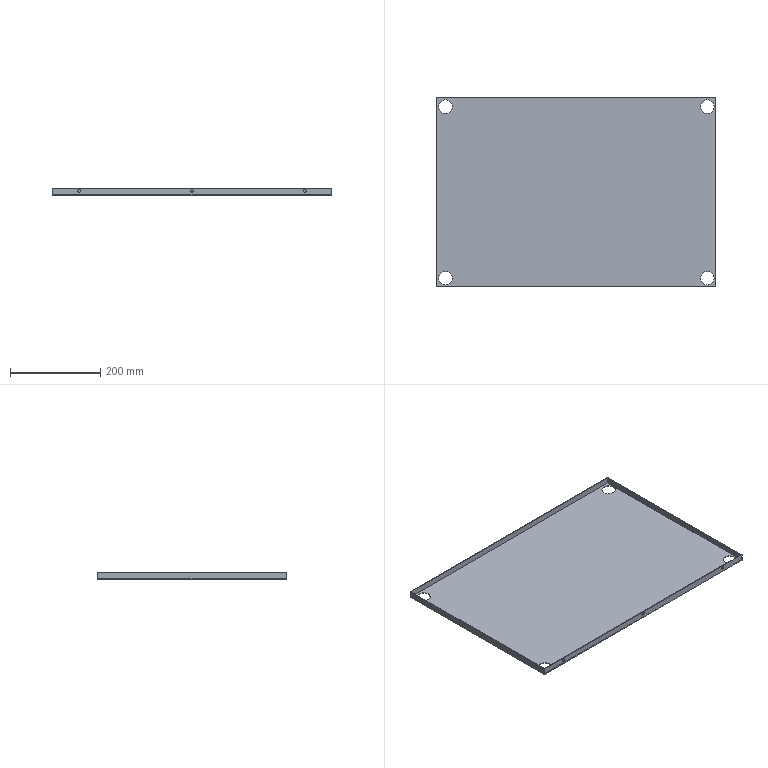Part | SolidWorks | features BaseBody 1 | 1 solid | 25 faces | box 620 x 420 x 15 mm | volume 428208 mm3 | cylinder 14 | plane 11 | commonest cylinder face diameters 30 x8 6.5 x6
STEP:
#1=CARTESIAN_POINT('',(437.517,75.647,0.));
#2=VERTEX_POINT('',#1);
#3=CARTESIAN_POINT('',(467.517,75.647,0.));
#4=VERTEX_POINT('',#3);
#5=CARTESIAN_POINT('',(452.517,75.647,0.));
#6=DIRECTION('',(0.,0.,1.));
#7=DIRECTION('',(1.,0.,0.));
#8=AXIS2_PLACEMENT_3D('',#5,#6,#7);
#9=CIRCLE('',#8,15.);
#10=EDGE_CURVE('',#2,#4,#9,.T.);
#11=ORIENTED_EDGE('',*,*,#10,.F.);
#12=CARTESIAN_POINT('',(437.517,75.647,1.5));
#13=VERTEX_POINT('',#12);
#14=CARTESIAN_POINT('',(437.517,75.647,0.));
#15=DIRECTION('',(0.,0.,1.));
#16=VECTOR('',#15,1000.);
#17=LINE('',#14,#16);
#18=EDGE_CURVE('',#2,#13,#17,.T.);
#19=ORIENTED_EDGE('',*,*,#18,.T.);
#20=CARTESIAN_POINT('',(467.517,75.647,1.5));
#21=VERTEX_POINT('',#20);
#22=CARTESIAN_POINT('',(452.517,75.647,1.5));
#23=DIRECTION('',(0.,0.,-1.));
#24=DIRECTION('',(1.,0.,0.));
#25=AXIS2_PLACEMENT_3D('',#22,#23,#24);
#26=CIRCLE('',#25,15.);
#27=EDGE_CURVE('',#21,#13,#26,.T.);
#28=ORIENTED_EDGE('',*,*,#27,.F.);
#29=CARTESIAN_POINT('',(467.517,75.647,0.));
#30=DIRECTION('',(0.,0.,1.));
#31=VECTOR('',#30,1000.);
#32=LINE('',#29,#31);
#33=EDGE_CURVE('',#4,#21,#32,.T.);
#34=ORIENTED_EDGE('',*,*,#33,.F.);
#35=EDGE_LOOP('',(#11,#19,#28,#34));
#36=FACE_OUTER_BOUND('',#35,.T.);
#37=CARTESIAN_POINT('',(452.517,75.647,0.));
#38=DIRECTION('',(0.,0.,1.));
#39=DIRECTION('',(1.,0.,0.));
#40=AXIS2_PLACEMENT_3D('',#37,#38,#39);
#41=CYLINDRICAL_SURFACE('',#40,15.);
#42=ADVANCED_FACE('',(#36),#41,.F.);
#43=CARTESIAN_POINT('',(-142.483,75.647,0.));
#44=VERTEX_POINT('',#43);
#45=CARTESIAN_POINT('',(-112.483,75.647,0.));
#46=VERTEX_POINT('',#45);
#47=CARTESIAN_POINT('',(-127.483,75.647,0.));
#48=DIRECTION('',(0.,0.,1.));
#49=DIRECTION('',(1.,0.,0.));
#50=AXIS2_PLACEMENT_3D('',#47,#48,#49);
#51=CIRCLE('',#50,15.);
#52=EDGE_CURVE('',#44,#46,#51,.T.);
#53=ORIENTED_EDGE('',*,*,#52,.F.);
#54=CARTESIAN_POINT('',(-142.483,75.647,1.5));
#55=VERTEX_POINT('',#54);
#56=CARTESIAN_POINT('',(-142.483,75.647,0.));
#57=DIRECTION('',(0.,0.,1.));
#58=VECTOR('',#57,1000.);
#59=LINE('',#56,#58);
#60=EDGE_CURVE('',#44,#55,#59,.T.);
#61=ORIENTED_EDGE('',*,*,#60,.T.);
#62=CARTESIAN_POINT('',(-112.483,75.647,1.5));
#63=VERTEX_POINT('',#62);
#64=CARTESIAN_POINT('',(-127.483,75.647,1.5));
#65=DIRECTION('',(0.,0.,-1.));
#66=DIRECTION('',(1.,0.,0.));
#67=AXIS2_PLACEMENT_3D('',#64,#65,#66);
#68=CIRCLE('',#67,15.);
#69=EDGE_CURVE('',#63,#55,#68,.T.);
#70=ORIENTED_EDGE('',*,*,#69,.F.);
#71=CARTESIAN_POINT('',(-112.483,75.647,0.));
#72=DIRECTION('',(0.,0.,1.));
#73=VECTOR('',#72,1000.);
#74=LINE('',#71,#73);
#75=EDGE_CURVE('',#46,#63,#74,.T.);
#76=ORIENTED_EDGE('',*,*,#75,.F.);
#77=EDGE_LOOP('',(#53,#61,#70,#76));
#78=FACE_OUTER_BOUND('',#77,.T.);
#79=CARTESIAN_POINT('',(-127.483,75.647,0.));
#80=DIRECTION('',(0.,0.,1.));
#81=DIRECTION('',(1.,0.,0.));
#82=AXIS2_PLACEMENT_3D('',#79,#80,#81);
#83=CYLINDRICAL_SURFACE('',#82,15.);
#84=ADVANCED_FACE('',(#78),#83,.F.);
#85=CARTESIAN_POINT('',(437.517,455.647,0.));
#86=VERTEX_POINT('',#85);
#87=CARTESIAN_POINT('',(467.517,455.647,0.));
#88=VERTEX_POINT('',#87);
#89=CARTESIAN_POINT('',(452.517,455.647,0.));
#90=DIRECTION('',(0.,0.,1.));
#91=DIRECTION('',(1.,0.,0.));
#92=AXIS2_PLACEMENT_3D('',#89,#90,#91);
#93=CIRCLE('',#92,15.);
#94=EDGE_CURVE('',#86,#88,#93,.T.);
#95=ORIENTED_EDGE('',*,*,#94,.F.);
#96=CARTESIAN_POINT('',(437.517,455.647,1.5));
#97=VERTEX_POINT('',#96);
#98=CARTESIAN_POINT('',(437.517,455.647,0.));
#99=DIRECTION('',(0.,0.,1.));
#100=VECTOR('',#99,1000.);
#101=LINE('',#98,#100);
#102=EDGE_CURVE('',#86,#97,#101,.T.);
#103=ORIENTED_EDGE('',*,*,#102,.T.);
#104=CARTESIAN_POINT('',(467.517,455.647,1.5));
#105=VERTEX_POINT('',#104);
#106=CARTESIAN_POINT('',(452.517,455.647,1.5));
#107=DIRECTION('',(0.,0.,-1.));
#108=DIRECTION('',(1.,0.,0.));
#109=AXIS2_PLACEMENT_3D('',#106,#107,#108);
#110=CIRCLE('',#109,15.);
#111=EDGE_CURVE('',#105,#97,#110,.T.);
#112=ORIENTED_EDGE('',*,*,#111,.F.);
#113=CARTESIAN_POINT('',(467.517,455.647,0.));
#114=DIRECTION('',(0.,0.,1.));
#115=VECTOR('',#114,1000.);
#116=LINE('',#113,#115);
#117=EDGE_CURVE('',#88,#105,#116,.T.);
#118=ORIENTED_EDGE('',*,*,#117,.F.);
#119=EDGE_LOOP('',(#95,#103,#112,#118));
#120=FACE_OUTER_BOUND('',#119,.T.);
#121=CARTESIAN_POINT('',(452.517,455.647,0.));
#122=DIRECTION('',(0.,0.,1.));
#123=DIRECTION('',(1.,0.,0.));
#124=AXIS2_PLACEMENT_3D('',#121,#122,#123);
#125=CYLINDRICAL_SURFACE('',#124,15.);
#126=ADVANCED_FACE('',(#120),#125,.F.);
#127=CARTESIAN_POINT('',(-142.483,455.647,0.));
#128=VERTEX_POINT('',#127);
#129=CARTESIAN_POINT('',(-112.483,455.647,0.));
#130=VERTEX_POINT('',#129);
#131=CARTESIAN_POINT('',(-127.483,455.647,0.));
#132=DIRECTION('',(0.,0.,1.));
#133=DIRECTION('',(1.,0.,0.));
#134=AXIS2_PLACEMENT_3D('',#131,#132,#133);
#135=CIRCLE('',#134,15.);
#136=EDGE_CURVE('',#128,#130,#135,.T.);
#137=ORIENTED_EDGE('',*,*,#136,.F.);
#138=CARTESIAN_POINT('',(-142.483,455.647,1.5));
#139=VERTEX_POINT('',#138);
#140=CARTESIAN_POINT('',(-142.483,455.647,0.));
#141=DIRECTION('',(0.,0.,1.));
#142=VECTOR('',#141,1000.);
#143=LINE('',#140,#142);
#144=EDGE_CURVE('',#128,#139,#143,.T.);
#145=ORIENTED_EDGE('',*,*,#144,.T.);
#146=CARTESIAN_POINT('',(-112.483,455.647,1.5));
#147=VERTEX_POINT('',#146);
#148=CARTESIAN_POINT('',(-127.483,455.647,1.5));
#149=DIRECTION('',(0.,0.,-1.));
#150=DIRECTION('',(1.,0.,0.));
#151=AXIS2_PLACEMENT_3D('',#148,#149,#150);
#152=CIRCLE('',#151,15.);
#153=EDGE_CURVE('',#147,#139,#152,.T.);
#154=ORIENTED_EDGE('',*,*,#153,.F.);
#155=CARTESIAN_POINT('',(-112.483,455.647,0.));
#156=DIRECTION('',(0.,0.,1.));
#157=VECTOR('',#156,1000.);
#158=LINE('',#155,#157);
#159=EDGE_CURVE('',#130,#147,#158,.T.);
#160=ORIENTED_EDGE('',*,*,#159,.F.);
#161=EDGE_LOOP('',(#137,#145,#154,#160));
#162=FACE_OUTER_BOUND('',#161,.T.);
#163=CARTESIAN_POINT('',(-127.483,455.647,0.));
#164=DIRECTION('',(0.,0.,1.));
#165=DIRECTION('',(1.,0.,0.));
#166=AXIS2_PLACEMENT_3D('',#163,#164,#165);
#167=CYLINDRICAL_SURFACE('',#166,15.);
#168=ADVANCED_FACE('',(#162),#167,.F.);
#169=CARTESIAN_POINT('',(411.517,58.147,13.25));
#170=VERTEX_POINT('',#169);
#171=CARTESIAN_POINT('',(411.517,58.147,6.75));
#172=VERTEX_POINT('',#171);
#173=CARTESIAN_POINT('',(411.517,58.147,10.));
#174=DIRECTION('',(0.,-1.,0.));
#175=DIRECTION('',(0.,0.,-1.));
#176=AXIS2_PLACEMENT_3D('',#173,#174,#175);
#177=CIRCLE('',#176,3.25);
#178=EDGE_CURVE('',#170,#172,#177,.T.);
#179=ORIENTED_EDGE('',*,*,#178,.F.);
#180=CARTESIAN_POINT('',(411.517,56.647,13.25));
#181=VERTEX_POINT('',#180);
#182=CARTESIAN_POINT('',(411.517,56.647,13.25));
#183=DIRECTION('',(0.,-1.,0.));
#184=VECTOR('',#183,1000.);
#185=LINE('',#182,#184);
#186=EDGE_CURVE('',#170,#181,#185,.T.);
#187=ORIENTED_EDGE('',*,*,#186,.T.);
#188=CARTESIAN_POINT('',(411.517,56.647,6.75));
#189=VERTEX_POINT('',#188);
#190=CARTESIAN_POINT('',(411.517,56.647,10.));
#191=DIRECTION('',(0.,-1.,0.));
#192=DIRECTION('',(0.,0.,-1.));
#193=AXIS2_PLACEMENT_3D('',#190,#191,#192);
#194=CIRCLE('',#193,3.25);
#195=EDGE_CURVE('',#181,#189,#194,.T.);
#196=ORIENTED_EDGE('',*,*,#195,.T.);
#197=CARTESIAN_POINT('',(411.517,56.647,6.75));
#198=DIRECTION('',(0.,-1.,0.));
#199=VECTOR('',#198,1000.);
#200=LINE('',#197,#199);
#201=EDGE_CURVE('',#172,#189,#200,.T.);
#202=ORIENTED_EDGE('',*,*,#201,.F.);
#203=EDGE_LOOP('',(#179,#187,#196,#202));
#204=FACE_OUTER_BOUND('',#203,.T.);
#205=CARTESIAN_POINT('',(411.517,56.647,10.));
#206=DIRECTION('',(0.,-1.,0.));
#207=DIRECTION('',(0.,0.,-1.));
#208=AXIS2_PLACEMENT_3D('',#205,#206,#207);
#209=CYLINDRICAL_SURFACE('',#208,3.25);
#210=ADVANCED_FACE('',(#204),#209,.F.);
#211=CARTESIAN_POINT('',(-88.483,58.147,13.25));
#212=VERTEX_POINT('',#211);
#213=CARTESIAN_POINT('',(-88.483,58.147,6.75));
#214=VERTEX_POINT('',#213);
#215=CARTESIAN_POINT('',(-88.483,58.147,10.));
#216=DIRECTION('',(0.,-1.,0.));
#217=DIRECTION('',(0.,0.,-1.));
#218=AXIS2_PLACEMENT_3D('',#215,#216,#217);
#219=CIRCLE('',#218,3.25);
#220=EDGE_CURVE('',#212,#214,#219,.T.);
#221=ORIENTED_EDGE('',*,*,#220,.F.);
#222=CARTESIAN_POINT('',(-88.483,56.647,13.25));
#223=VERTEX_POINT('',#222);
#224=CARTESIAN_POINT('',(-88.483,56.647,13.25));
#225=DIRECTION('',(0.,-1.,0.));
#226=VECTOR('',#225,1000.);
#227=LINE('',#224,#226);
#228=EDGE_CURVE('',#212,#223,#227,.T.);
#229=ORIENTED_EDGE('',*,*,#228,.T.);
#230=CARTESIAN_POINT('',(-88.483,56.647,6.75));
#231=VERTEX_POINT('',#230);
#232=CARTESIAN_POINT('',(-88.483,56.647,10.));
#233=DIRECTION('',(0.,-1.,0.));
#234=DIRECTION('',(0.,0.,-1.));
#235=AXIS2_PLACEMENT_3D('',#232,#233,#234);
#236=CIRCLE('',#235,3.25);
#237=EDGE_CURVE('',#223,#231,#236,.T.);
#238=ORIENTED_EDGE('',*,*,#237,.T.);
#239=CARTESIAN_POINT('',(-88.483,56.647,6.75));
#240=DIRECTION('',(0.,-1.,0.));
#241=VECTOR('',#240,1000.);
#242=LINE('',#239,#241);
#243=EDGE_CURVE('',#214,#231,#242,.T.);
#244=ORIENTED_EDGE('',*,*,#243,.F.);
#245=EDGE_LOOP('',(#221,#229,#238,#244));
#246=FACE_OUTER_BOUND('',#245,.T.);
#247=CARTESIAN_POINT('',(-88.483,56.647,10.));
#248=DIRECTION('',(0.,-1.,0.));
#249=DIRECTION('',(0.,0.,-1.));
#250=AXIS2_PLACEMENT_3D('',#247,#248,#249);
#251=CYLINDRICAL_SURFACE('',#250,3.25);
#252=ADVANCED_FACE('',(#246),#251,.F.);
#253=CARTESIAN_POINT('',(161.517,58.147,13.25));
#254=VERTEX_POINT('',#253);
#255=CARTESIAN_POINT('',(161.517,58.147,6.75));
#256=VERTEX_POINT('',#255);
#257=CARTESIAN_POINT('',(161.517,58.147,10.));
#258=DIRECTION('',(0.,-1.,0.));
#259=DIRECTION('',(0.,0.,-1.));
#260=AXIS2_PLACEMENT_3D('',#257,#258,#259);
#261=CIRCLE('',#260,3.25);
#262=EDGE_CURVE('',#254,#256,#261,.T.);
#263=ORIENTED_EDGE('',*,*,#262,.F.);
#264=CARTESIAN_POINT('',(161.517,56.647,13.25));
#265=VERTEX_POINT('',#264);
#266=CARTESIAN_POINT('',(161.517,56.647,13.25));
#267=DIRECTION('',(0.,-1.,0.));
#268=VECTOR('',#267,1000.);
#269=LINE('',#266,#268);
#270=EDGE_CURVE('',#254,#265,#269,.T.);
#271=ORIENTED_EDGE('',*,*,#270,.T.);
#272=CARTESIAN_POINT('',(161.517,56.647,6.75));
#273=VERTEX_POINT('',#272);
#274=CARTESIAN_POINT('',(161.517,56.647,10.));
#275=DIRECTION('',(0.,-1.,0.));
#276=DIRECTION('',(0.,0.,-1.));
#277=AXIS2_PLACEMENT_3D('',#274,#275,#276);
#278=CIRCLE('',#277,3.25);
#279=EDGE_CURVE('',#265,#273,#278,.T.);
#280=ORIENTED_EDGE('',*,*,#279,.T.);
#281=CARTESIAN_POINT('',(161.517,56.647,6.75));
#282=DIRECTION('',(0.,-1.,0.));
#283=VECTOR('',#282,1000.);
#284=LINE('',#281,#283);
#285=EDGE_CURVE('',#256,#273,#284,.T.);
#286=ORIENTED_EDGE('',*,*,#285,.F.);
#287=EDGE_LOOP('',(#263,#271,#280,#286));
#288=FACE_OUTER_BOUND('',#287,.T.);
#289=CARTESIAN_POINT('',(161.517,56.647,10.));
#290=DIRECTION('',(0.,-1.,0.));
#291=DIRECTION('',(0.,0.,-1.));
#292=AXIS2_PLACEMENT_3D('',#289,#290,#291);
#293=CYLINDRICAL_SURFACE('',#292,3.25);
#294=ADVANCED_FACE('',(#288),#293,.F.);
#295=CARTESIAN_POINT('',(-148.483,56.647,0.));
#296=VERTEX_POINT('',#295);
#297=CARTESIAN_POINT('',(-148.483,476.647,0.));
#298=VERTEX_POINT('',#297);
#299=CARTESIAN_POINT('',(-148.483,0.,0.));
#300=DIRECTION('',(0.,1.,0.));
#301=VECTOR('',#300,1000.);
#302=LINE('',#299,#301);
#303=EDGE_CURVE('',#296,#298,#302,.T.);
#304=ORIENTED_EDGE('',*,*,#303,.T.);
#305=CARTESIAN_POINT('',(471.517,476.647,0.));
#306=VERTEX_POINT('',#305);
#307=CARTESIAN_POINT('',(0.,476.647,0.));
#308=DIRECTION('',(1.,0.,0.));
#309=VECTOR('',#308,1000.);
#310=LINE('',#307,#309);
#311=EDGE_CURVE('',#298,#306,#310,.T.);
#312=ORIENTED_EDGE('',*,*,#311,.T.);
#313=CARTESIAN_POINT('',(471.517,56.647,0.));
#314=VERTEX_POINT('',#313);
#315=CARTESIAN_POINT('',(471.517,0.,0.));
#316=DIRECTION('',(0.,-1.,0.));
#317=VECTOR('',#316,1000.);
#318=LINE('',#315,#317);
#319=EDGE_CURVE('',#306,#314,#318,.T.);
#320=ORIENTED_EDGE('',*,*,#319,.T.);
#321=CARTESIAN_POINT('',(0.,56.647,0.));
#322=DIRECTION('',(-1.,0.,0.));
#323=VECTOR('',#322,1000.);
#324=LINE('',#321,#323);
#325=EDGE_CURVE('',#314,#296,#324,.T.);
#326=ORIENTED_EDGE('',*,*,#325,.T.);
#327=EDGE_LOOP('',(#304,#312,#320,#326));
#328=FACE_OUTER_BOUND('',#327,.T.);
#329=CARTESIAN_POINT('',(452.517,75.647,0.));
#330=DIRECTION('',(0.,0.,1.));
#331=DIRECTION('',(1.,0.,0.));
#332=AXIS2_PLACEMENT_3D('',#329,#330,#331);
#333=CIRCLE('',#332,15.);
#334=EDGE_CURVE('',#4,#2,#333,.T.);
#335=ORIENTED_EDGE('',*,*,#334,.T.);
#336=ORIENTED_EDGE('',*,*,#10,.T.);
#337=EDGE_LOOP('',(#335,#336));
#338=FACE_BOUND('',#337,.T.);
#339=CARTESIAN_POINT('',(-127.483,75.647,0.));
#340=DIRECTION('',(0.,0.,1.));
#341=DIRECTION('',(1.,0.,0.));
#342=AXIS2_PLACEMENT_3D('',#339,#340,#341);
#343=CIRCLE('',#342,15.);
#344=EDGE_CURVE('',#46,#44,#343,.T.);
#345=ORIENTED_EDGE('',*,*,#344,.T.);
#346=ORIENTED_EDGE('',*,*,#52,.T.);
#347=EDGE_LOOP('',(#345,#346));
#348=FACE_BOUND('',#347,.T.);
#349=CARTESIAN_POINT('',(452.517,455.647,0.));
#350=DIRECTION('',(0.,0.,1.));
#351=DIRECTION('',(1.,0.,0.));
#352=AXIS2_PLACEMENT_3D('',#349,#350,#351);
#353=CIRCLE('',#352,15.);
#354=EDGE_CURVE('',#88,#86,#353,.T.);
#355=ORIENTED_EDGE('',*,*,#354,.T.);
#356=ORIENTED_EDGE('',*,*,#94,.T.);
#357=EDGE_LOOP('',(#355,#356));
#358=FACE_BOUND('',#357,.T.);
#359=CARTESIAN_POINT('',(-127.483,455.647,0.));
#360=DIRECTION('',(0.,0.,1.));
#361=DIRECTION('',(1.,0.,0.));
#362=AXIS2_PLACEMENT_3D('',#359,#360,#361);
#363=CIRCLE('',#362,15.);
#364=EDGE_CURVE('',#130,#128,#363,.T.);
#365=ORIENTED_EDGE('',*,*,#364,.T.);
#366=ORIENTED_EDGE('',*,*,#136,.T.);
#367=EDGE_LOOP('',(#365,#366));
#368=FACE_BOUND('',#367,.T.);
#369=CARTESIAN_POINT('',(0.,0.,0.));
#370=DIRECTION('',(0.,0.,-1.));
#371=DIRECTION('',(-1.,0.,0.));
#372=AXIS2_PLACEMENT_3D('',#369,#370,#371);
#373=PLANE('',#372);
#374=ADVANCED_FACE('',(#328,#338,#348,#358,#368),#373,.T.);
#375=CARTESIAN_POINT('',(-148.483,476.647,15.));
#376=VERTEX_POINT('',#375);
#377=CARTESIAN_POINT('',(-148.483,476.647,15.));
#378=DIRECTION('',(0.,0.,-1.));
#379=VECTOR('',#378,1000.);
#380=LINE('',#377,#379);
#381=EDGE_CURVE('',#376,#298,#380,.T.);
#382=ORIENTED_EDGE('',*,*,#381,.F.);
#383=CARTESIAN_POINT('',(471.517,476.647,15.));
#384=VERTEX_POINT('',#383);
#385=CARTESIAN_POINT('',(471.517,476.647,15.));
#386=DIRECTION('',(-1.,0.,0.));
#387=VECTOR('',#386,1000.);
#388=LINE('',#385,#387);
#389=EDGE_CURVE('',#384,#376,#388,.T.);
#390=ORIENTED_EDGE('',*,*,#389,.F.);
#391=CARTESIAN_POINT('',(471.517,476.647,15.));
#392=DIRECTION('',(0.,0.,1.));
#393=VECTOR('',#392,1000.);
#394=LINE('',#391,#393);
#395=EDGE_CURVE('',#306,#384,#394,.T.);
#396=ORIENTED_EDGE('',*,*,#395,.F.);
#397=ORIENTED_EDGE('',*,*,#311,.F.);
#398=EDGE_LOOP('',(#382,#390,#396,#397));
#399=FACE_OUTER_BOUND('',#398,.T.);
#400=CARTESIAN_POINT('',(471.517,476.647,15.));
#401=DIRECTION('',(0.,-1.,0.));
#402=DIRECTION('',(1.,0.,0.));
#403=AXIS2_PLACEMENT_3D('',#400,#401,#402);
#404=PLANE('',#403);
#405=ADVANCED_FACE('',(#399),#404,.F.);
#406=CARTESIAN_POINT('',(-148.483,56.647,15.));
#407=VERTEX_POINT('',#406);
#408=CARTESIAN_POINT('',(-148.483,56.647,15.));
#409=DIRECTION('',(0.,0.,-1.));
#410=VECTOR('',#409,1000.);
#411=LINE('',#408,#410);
#412=EDGE_CURVE('',#407,#296,#411,.T.);
#413=ORIENTED_EDGE('',*,*,#412,.F.);
#414=CARTESIAN_POINT('',(-148.483,476.647,15.));
#415=DIRECTION('',(0.,-1.,0.));
#416=VECTOR('',#415,1000.);
#417=LINE('',#414,#416);
#418=EDGE_CURVE('',#376,#407,#417,.T.);
#419=ORIENTED_EDGE('',*,*,#418,.F.);
#420=ORIENTED_EDGE('',*,*,#381,.T.);
#421=ORIENTED_EDGE('',*,*,#303,.F.);
#422=EDGE_LOOP('',(#413,#419,#420,#421));
#423=FACE_OUTER_BOUND('',#422,.T.);
#424=CARTESIAN_POINT('',(-148.483,476.647,15.));
#425=DIRECTION('',(1.,0.,0.));
#426=DIRECTION('',(0.,0.,-1.));
#427=AXIS2_PLACEMENT_3D('',#424,#425,#426);
#428=PLANE('',#427);
#429=ADVANCED_FACE('',(#423),#428,.F.);
#430=CARTESIAN_POINT('',(471.517,56.647,15.));
#431=VERTEX_POINT('',#430);
#432=CARTESIAN_POINT('',(471.517,56.647,15.));
#433=DIRECTION('',(0.,0.,-1.));
#434=VECTOR('',#433,1000.);
#435=LINE('',#432,#434);
#436=EDGE_CURVE('',#431,#314,#435,.T.);
#437=ORIENTED_EDGE('',*,*,#436,.F.);
#438=CARTESIAN_POINT('',(471.517,56.647,15.));
#439=DIRECTION('',(1.,0.,0.));
#440=VECTOR('',#439,1000.);
#441=LINE('',#438,#440);
#442=EDGE_CURVE('',#407,#431,#441,.T.);
#443=ORIENTED_EDGE('',*,*,#442,.F.);
#444=ORIENTED_EDGE('',*,*,#412,.T.);
#445=ORIENTED_EDGE('',*,*,#325,.F.);
#446=EDGE_LOOP('',(#437,#443,#444,#445));
#447=FACE_OUTER_BOUND('',#446,.T.);
#448=CARTESIAN_POINT('',(411.517,56.647,10.));
#449=DIRECTION('',(0.,-1.,0.));
#450=DIRECTION('',(0.,0.,-1.));
#451=AXIS2_PLACEMENT_3D('',#448,#449,#450);
#452=CIRCLE('',#451,3.25);
#453=EDGE_CURVE('',#189,#181,#452,.T.);
#454=ORIENTED_EDGE('',*,*,#453,.F.);
#455=ORIENTED_EDGE('',*,*,#195,.F.);
#456=EDGE_LOOP('',(#454,#455));
#457=FACE_BOUND('',#456,.T.);
#458=CARTESIAN_POINT('',(-88.483,56.647,10.));
#459=DIRECTION('',(0.,-1.,0.));
#460=DIRECTION('',(0.,0.,-1.));
#461=AXIS2_PLACEMENT_3D('',#458,#459,#460);
#462=CIRCLE('',#461,3.25);
#463=EDGE_CURVE('',#231,#223,#462,.T.);
#464=ORIENTED_EDGE('',*,*,#463,.F.);
#465=ORIENTED_EDGE('',*,*,#237,.F.);
#466=EDGE_LOOP('',(#464,#465));
#467=FACE_BOUND('',#466,.T.);
#468=CARTESIAN_POINT('',(161.517,56.647,10.));
#469=DIRECTION('',(0.,-1.,0.));
#470=DIRECTION('',(0.,0.,-1.));
#471=AXIS2_PLACEMENT_3D('',#468,#469,#470);
#472=CIRCLE('',#471,3.25);
#473=EDGE_CURVE('',#273,#265,#472,.T.);
#474=ORIENTED_EDGE('',*,*,#473,.F.);
#475=ORIENTED_EDGE('',*,*,#279,.F.);
#476=EDGE_LOOP('',(#474,#475));
#477=FACE_BOUND('',#476,.T.);
#478=CARTESIAN_POINT('',(471.517,56.647,15.));
#479=DIRECTION('',(0.,1.,0.));
#480=DIRECTION('',(-1.,0.,0.));
#481=AXIS2_PLACEMENT_3D('',#478,#479,#480);
#482=PLANE('',#481);
#483=ADVANCED_FACE('',(#447,#457,#467,#477),#482,.F.);
#484=ORIENTED_EDGE('',*,*,#395,.T.);
#485=CARTESIAN_POINT('',(471.517,476.647,15.));
#486=DIRECTION('',(0.,1.,0.));
#487=VECTOR('',#486,1000.);
#488=LINE('',#485,#487);
#489=EDGE_CURVE('',#431,#384,#488,.T.);
#490=ORIENTED_EDGE('',*,*,#489,.F.);
#491=ORIENTED_EDGE('',*,*,#436,.T.);
#492=ORIENTED_EDGE('',*,*,#319,.F.);
#493=EDGE_LOOP('',(#484,#490,#491,#492));
#494=FACE_OUTER_BOUND('',#493,.T.);
#495=CARTESIAN_POINT('',(471.517,476.647,15.));
#496=DIRECTION('',(-1.,0.,0.));
#497=DIRECTION('',(0.,-1.,0.));
#498=AXIS2_PLACEMENT_3D('',#495,#496,#497);
#499=PLANE('',#498);
#500=ADVANCED_FACE('',(#494),#499,.F.);
#501=ORIENTED_EDGE('',*,*,#18,.F.);
#502=ORIENTED_EDGE('',*,*,#334,.F.);
#503=ORIENTED_EDGE('',*,*,#33,.T.);
#504=CARTESIAN_POINT('',(452.517,75.647,1.5));
#505=DIRECTION('',(0.,0.,-1.));
#506=DIRECTION('',(1.,0.,0.));
#507=AXIS2_PLACEMENT_3D('',#504,#505,#506);
#508=CIRCLE('',#507,15.);
#509=EDGE_CURVE('',#13,#21,#508,.T.);
#510=ORIENTED_EDGE('',*,*,#509,.F.);
#511=EDGE_LOOP('',(#501,#502,#503,#510));
#512=FACE_OUTER_BOUND('',#511,.T.);
#513=CARTESIAN_POINT('',(452.517,75.647,0.));
#514=DIRECTION('',(0.,0.,1.));
#515=DIRECTION('',(1.,0.,0.));
#516=AXIS2_PLACEMENT_3D('',#513,#514,#515);
#517=CYLINDRICAL_SURFACE('',#516,15.);
#518=ADVANCED_FACE('',(#512),#517,.F.);
#519=ORIENTED_EDGE('',*,*,#60,.F.);
#520=ORIENTED_EDGE('',*,*,#344,.F.);
#521=ORIENTED_EDGE('',*,*,#75,.T.);
#522=CARTESIAN_POINT('',(-127.483,75.647,1.5));
#523=DIRECTION('',(0.,0.,-1.));
#524=DIRECTION('',(1.,0.,0.));
#525=AXIS2_PLACEMENT_3D('',#522,#523,#524);
#526=CIRCLE('',#525,15.);
#527=EDGE_CURVE('',#55,#63,#526,.T.);
#528=ORIENTED_EDGE('',*,*,#527,.F.);
#529=EDGE_LOOP('',(#519,#520,#521,#528));
#530=FACE_OUTER_BOUND('',#529,.T.);
#531=CARTESIAN_POINT('',(-127.483,75.647,0.));
#532=DIRECTION('',(0.,0.,1.));
#533=DIRECTION('',(1.,0.,0.));
#534=AXIS2_PLACEMENT_3D('',#531,#532,#533);
#535=CYLINDRICAL_SURFACE('',#534,15.);
#536=ADVANCED_FACE('',(#530),#535,.F.);
#537=ORIENTED_EDGE('',*,*,#102,.F.);
#538=ORIENTED_EDGE('',*,*,#354,.F.);
#539=ORIENTED_EDGE('',*,*,#117,.T.);
#540=CARTESIAN_POINT('',(452.517,455.647,1.5));
#541=DIRECTION('',(0.,0.,-1.));
#542=DIRECTION('',(1.,0.,0.));
#543=AXIS2_PLACEMENT_3D('',#540,#541,#542);
#544=CIRCLE('',#543,15.);
#545=EDGE_CURVE('',#97,#105,#544,.T.);
#546=ORIENTED_EDGE('',*,*,#545,.F.);
#547=EDGE_LOOP('',(#537,#538,#539,#546));
#548=FACE_OUTER_BOUND('',#547,.T.);
#549=CARTESIAN_POINT('',(452.517,455.647,0.));
#550=DIRECTION('',(0.,0.,1.));
#551=DIRECTION('',(1.,0.,0.));
#552=AXIS2_PLACEMENT_3D('',#549,#550,#551);
#553=CYLINDRICAL_SURFACE('',#552,15.);
#554=ADVANCED_FACE('',(#548),#553,.F.);
#555=ORIENTED_EDGE('',*,*,#144,.F.);
#556=ORIENTED_EDGE('',*,*,#364,.F.);
#557=ORIENTED_EDGE('',*,*,#159,.T.);
#558=CARTESIAN_POINT('',(-127.483,455.647,1.5));
#559=DIRECTION('',(0.,0.,-1.));
#560=DIRECTION('',(1.,0.,0.));
#561=AXIS2_PLACEMENT_3D('',#558,#559,#560);
#562=CIRCLE('',#561,15.);
#563=EDGE_CURVE('',#139,#147,#562,.T.);
#564=ORIENTED_EDGE('',*,*,#563,.F.);
#565=EDGE_LOOP('',(#555,#556,#557,#564));
#566=FACE_OUTER_BOUND('',#565,.T.);
#567=CARTESIAN_POINT('',(-127.483,455.647,0.));
#568=DIRECTION('',(0.,0.,1.));
#569=DIRECTION('',(1.,0.,0.));
#570=AXIS2_PLACEMENT_3D('',#567,#568,#569);
#571=CYLINDRICAL_SURFACE('',#570,15.);
#572=ADVANCED_FACE('',(#566),#571,.F.);
#573=CARTESIAN_POINT('',(-146.983,58.147,15.));
#574=VERTEX_POINT('',#573);
#575=CARTESIAN_POINT('',(470.017,58.147,15.));
#576=VERTEX_POINT('',#575);
#577=CARTESIAN_POINT('',(0.,58.147,15.));
#578=DIRECTION('',(1.,0.,0.));
#579=VECTOR('',#578,1000.);
#580=LINE('',#577,#579);
#581=EDGE_CURVE('',#574,#576,#580,.T.);
#582=ORIENTED_EDGE('',*,*,#581,.F.);
#583=CARTESIAN_POINT('',(-146.983,475.147,15.));
#584=VERTEX_POINT('',#583);
#585=CARTESIAN_POINT('',(-146.983,0.,15.));
#586=DIRECTION('',(0.,-1.,0.));
#587=VECTOR('',#586,1000.);
#588=LINE('',#585,#587);
#589=EDGE_CURVE('',#584,#574,#588,.T.);
#590=ORIENTED_EDGE('',*,*,#589,.F.);
#591=CARTESIAN_POINT('',(470.017,475.147,15.));
#592=VERTEX_POINT('',#591);
#593=CARTESIAN_POINT('',(0.,475.147,15.));
#594=DIRECTION('',(-1.,0.,0.));
#595=VECTOR('',#594,1000.);
#596=LINE('',#593,#595);
#597=EDGE_CURVE('',#592,#584,#596,.T.);
#598=ORIENTED_EDGE('',*,*,#597,.F.);
#599=CARTESIAN_POINT('',(470.017,0.,15.));
#600=DIRECTION('',(0.,1.,0.));
#601=VECTOR('',#600,1000.);
#602=LINE('',#599,#601);
#603=EDGE_CURVE('',#576,#592,#602,.T.);
#604=ORIENTED_EDGE('',*,*,#603,.F.);
#605=EDGE_LOOP('',(#582,#590,#598,#604));
#606=FACE_BOUND('',#605,.T.);
#607=ORIENTED_EDGE('',*,*,#389,.T.);
#608=ORIENTED_EDGE('',*,*,#418,.T.);
#609=ORIENTED_EDGE('',*,*,#442,.T.);
#610=ORIENTED_EDGE('',*,*,#489,.T.);
#611=EDGE_LOOP('',(#607,#608,#609,#610));
#612=FACE_OUTER_BOUND('',#611,.T.);
#613=CARTESIAN_POINT('',(0.,0.,15.));
#614=DIRECTION('',(0.,0.,-1.));
#615=DIRECTION('',(-1.,0.,0.));
#616=AXIS2_PLACEMENT_3D('',#613,#614,#615);
#617=PLANE('',#616);
#618=ADVANCED_FACE('',(#606,#612),#617,.F.);
#619=ORIENTED_EDGE('',*,*,#186,.F.);
#620=CARTESIAN_POINT('',(411.517,58.147,10.));
#621=DIRECTION('',(0.,-1.,0.));
#622=DIRECTION('',(0.,0.,-1.));
#623=AXIS2_PLACEMENT_3D('',#620,#621,#622);
#624=CIRCLE('',#623,3.25);
#625=EDGE_CURVE('',#172,#170,#624,.T.);
#626=ORIENTED_EDGE('',*,*,#625,.F.);
#627=ORIENTED_EDGE('',*,*,#201,.T.);
#628=ORIENTED_EDGE('',*,*,#453,.T.);
#629=EDGE_LOOP('',(#619,#626,#627,#628));
#630=FACE_OUTER_BOUND('',#629,.T.);
#631=CARTESIAN_POINT('',(411.517,56.647,10.));
#632=DIRECTION('',(0.,-1.,0.));
#633=DIRECTION('',(0.,0.,-1.));
#634=AXIS2_PLACEMENT_3D('',#631,#632,#633);
#635=CYLINDRICAL_SURFACE('',#634,3.25);
#636=ADVANCED_FACE('',(#630),#635,.F.);
#637=ORIENTED_EDGE('',*,*,#228,.F.);
#638=CARTESIAN_POINT('',(-88.483,58.147,10.));
#639=DIRECTION('',(0.,-1.,0.));
#640=DIRECTION('',(0.,0.,-1.));
#641=AXIS2_PLACEMENT_3D('',#638,#639,#640);
#642=CIRCLE('',#641,3.25);
#643=EDGE_CURVE('',#214,#212,#642,.T.);
#644=ORIENTED_EDGE('',*,*,#643,.F.);
#645=ORIENTED_EDGE('',*,*,#243,.T.);
#646=ORIENTED_EDGE('',*,*,#463,.T.);
#647=EDGE_LOOP('',(#637,#644,#645,#646));
#648=FACE_OUTER_BOUND('',#647,.T.);
#649=CARTESIAN_POINT('',(-88.483,56.647,10.));
#650=DIRECTION('',(0.,-1.,0.));
#651=DIRECTION('',(0.,0.,-1.));
#652=AXIS2_PLACEMENT_3D('',#649,#650,#651);
#653=CYLINDRICAL_SURFACE('',#652,3.25);
#654=ADVANCED_FACE('',(#648),#653,.F.);
#655=ORIENTED_EDGE('',*,*,#270,.F.);
#656=CARTESIAN_POINT('',(161.517,58.147,10.));
#657=DIRECTION('',(0.,-1.,0.));
#658=DIRECTION('',(0.,0.,-1.));
#659=AXIS2_PLACEMENT_3D('',#656,#657,#658);
#660=CIRCLE('',#659,3.25);
#661=EDGE_CURVE('',#256,#254,#660,.T.);
#662=ORIENTED_EDGE('',*,*,#661,.F.);
#663=ORIENTED_EDGE('',*,*,#285,.T.);
#664=ORIENTED_EDGE('',*,*,#473,.T.);
#665=EDGE_LOOP('',(#655,#662,#663,#664));
#666=FACE_OUTER_BOUND('',#665,.T.);
#667=CARTESIAN_POINT('',(161.517,56.647,10.));
#668=DIRECTION('',(0.,-1.,0.));
#669=DIRECTION('',(0.,0.,-1.));
#670=AXIS2_PLACEMENT_3D('',#667,#668,#669);
#671=CYLINDRICAL_SURFACE('',#670,3.25);
#672=ADVANCED_FACE('',(#666),#671,.F.);
#673=CARTESIAN_POINT('',(-146.983,475.147,1.5));
#674=VERTEX_POINT('',#673);
#675=CARTESIAN_POINT('',(470.017,475.147,1.5));
#676=VERTEX_POINT('',#675);
#677=CARTESIAN_POINT('',(0.,475.147,1.5));
#678=DIRECTION('',(1.,0.,0.));
#679=VECTOR('',#678,1000.);
#680=LINE('',#677,#679);
#681=EDGE_CURVE('',#674,#676,#680,.T.);
#682=ORIENTED_EDGE('',*,*,#681,.F.);
#683=CARTESIAN_POINT('',(-146.983,58.147,1.5));
#684=VERTEX_POINT('',#683);
#685=CARTESIAN_POINT('',(-146.983,0.,1.5));
#686=DIRECTION('',(0.,1.,0.));
#687=VECTOR('',#686,1000.);
#688=LINE('',#685,#687);
#689=EDGE_CURVE('',#684,#674,#688,.T.);
#690=ORIENTED_EDGE('',*,*,#689,.F.);
#691=CARTESIAN_POINT('',(470.017,58.147,1.5));
#692=VERTEX_POINT('',#691);
#693=CARTESIAN_POINT('',(0.,58.147,1.5));
#694=DIRECTION('',(-1.,0.,0.));
#695=VECTOR('',#694,1000.);
#696=LINE('',#693,#695);
#697=EDGE_CURVE('',#692,#684,#696,.T.);
#698=ORIENTED_EDGE('',*,*,#697,.F.);
#699=CARTESIAN_POINT('',(470.017,0.,1.5));
#700=DIRECTION('',(0.,-1.,0.));
#701=VECTOR('',#700,1000.);
#702=LINE('',#699,#701);
#703=EDGE_CURVE('',#676,#692,#702,.T.);
#704=ORIENTED_EDGE('',*,*,#703,.F.);
#705=EDGE_LOOP('',(#682,#690,#698,#704));
#706=FACE_OUTER_BOUND('',#705,.T.);
#707=ORIENTED_EDGE('',*,*,#27,.T.);
#708=ORIENTED_EDGE('',*,*,#509,.T.);
#709=EDGE_LOOP('',(#707,#708));
#710=FACE_BOUND('',#709,.T.);
#711=ORIENTED_EDGE('',*,*,#69,.T.);
#712=ORIENTED_EDGE('',*,*,#527,.T.);
#713=EDGE_LOOP('',(#711,#712));
#714=FACE_BOUND('',#713,.T.);
#715=ORIENTED_EDGE('',*,*,#111,.T.);
#716=ORIENTED_EDGE('',*,*,#545,.T.);
#717=EDGE_LOOP('',(#715,#716));
#718=FACE_BOUND('',#717,.T.);
#719=ORIENTED_EDGE('',*,*,#153,.T.);
#720=ORIENTED_EDGE('',*,*,#563,.T.);
#721=EDGE_LOOP('',(#719,#720));
#722=FACE_BOUND('',#721,.T.);
#723=CARTESIAN_POINT('',(0.,0.,1.5));
#724=DIRECTION('',(0.,0.,-1.));
#725=DIRECTION('',(-1.,0.,0.));
#726=AXIS2_PLACEMENT_3D('',#723,#724,#725);
#727=PLANE('',#726);
#728=ADVANCED_FACE('',(#706,#710,#714,#718,#722),#727,.F.);
#729=ORIENTED_EDGE('',*,*,#603,.T.);
#730=CARTESIAN_POINT('',(470.017,475.147,15.));
#731=DIRECTION('',(0.,0.,-1.));
#732=VECTOR('',#731,1000.);
#733=LINE('',#730,#732);
#734=EDGE_CURVE('',#592,#676,#733,.T.);
#735=ORIENTED_EDGE('',*,*,#734,.T.);
#736=ORIENTED_EDGE('',*,*,#703,.T.);
#737=CARTESIAN_POINT('',(470.017,58.147,15.));
#738=DIRECTION('',(0.,0.,1.));
#739=VECTOR('',#738,1000.);
#740=LINE('',#737,#739);
#741=EDGE_CURVE('',#692,#576,#740,.T.);
#742=ORIENTED_EDGE('',*,*,#741,.T.);
#743=EDGE_LOOP('',(#729,#735,#736,#742));
#744=FACE_OUTER_BOUND('',#743,.T.);
#745=CARTESIAN_POINT('',(470.017,476.647,15.));
#746=DIRECTION('',(-1.,0.,0.));
#747=DIRECTION('',(0.,-1.,0.));
#748=AXIS2_PLACEMENT_3D('',#745,#746,#747);
#749=PLANE('',#748);
#750=ADVANCED_FACE('',(#744),#749,.T.);
#751=ORIENTED_EDGE('',*,*,#581,.T.);
#752=ORIENTED_EDGE('',*,*,#741,.F.);
#753=ORIENTED_EDGE('',*,*,#697,.T.);
#754=CARTESIAN_POINT('',(-146.983,58.147,15.));
#755=DIRECTION('',(0.,0.,1.));
#756=VECTOR('',#755,1000.);
#757=LINE('',#754,#756);
#758=EDGE_CURVE('',#684,#574,#757,.T.);
#759=ORIENTED_EDGE('',*,*,#758,.T.);
#760=EDGE_LOOP('',(#751,#752,#753,#759));
#761=FACE_OUTER_BOUND('',#760,.T.);
#762=ORIENTED_EDGE('',*,*,#625,.T.);
#763=ORIENTED_EDGE('',*,*,#178,.T.);
#764=EDGE_LOOP('',(#762,#763));
#765=FACE_BOUND('',#764,.T.);
#766=ORIENTED_EDGE('',*,*,#643,.T.);
#767=ORIENTED_EDGE('',*,*,#220,.T.);
#768=EDGE_LOOP('',(#766,#767));
#769=FACE_BOUND('',#768,.T.);
#770=ORIENTED_EDGE('',*,*,#661,.T.);
#771=ORIENTED_EDGE('',*,*,#262,.T.);
#772=EDGE_LOOP('',(#770,#771));
#773=FACE_BOUND('',#772,.T.);
#774=CARTESIAN_POINT('',(471.517,58.147,15.));
#775=DIRECTION('',(0.,1.,0.));
#776=DIRECTION('',(-1.,0.,0.));
#777=AXIS2_PLACEMENT_3D('',#774,#775,#776);
#778=PLANE('',#777);
#779=ADVANCED_FACE('',(#761,#765,#769,#773),#778,.T.);
#780=ORIENTED_EDGE('',*,*,#589,.T.);
#781=ORIENTED_EDGE('',*,*,#758,.F.);
#782=ORIENTED_EDGE('',*,*,#689,.T.);
#783=CARTESIAN_POINT('',(-146.983,475.147,15.));
#784=DIRECTION('',(0.,0.,1.));
#785=VECTOR('',#784,1000.);
#786=LINE('',#783,#785);
#787=EDGE_CURVE('',#674,#584,#786,.T.);
#788=ORIENTED_EDGE('',*,*,#787,.T.);
#789=EDGE_LOOP('',(#780,#781,#782,#788));
#790=FACE_OUTER_BOUND('',#789,.T.);
#791=CARTESIAN_POINT('',(-146.983,476.647,15.));
#792=DIRECTION('',(1.,0.,0.));
#793=DIRECTION('',(0.,0.,-1.));
#794=AXIS2_PLACEMENT_3D('',#791,#792,#793);
#795=PLANE('',#794);
#796=ADVANCED_FACE('',(#790),#795,.T.);
#797=ORIENTED_EDGE('',*,*,#597,.T.);
#798=ORIENTED_EDGE('',*,*,#787,.F.);
#799=ORIENTED_EDGE('',*,*,#681,.T.);
#800=ORIENTED_EDGE('',*,*,#734,.F.);
#801=EDGE_LOOP('',(#797,#798,#799,#800));
#802=FACE_OUTER_BOUND('',#801,.T.);
#803=CARTESIAN_POINT('',(471.517,475.147,15.));
#804=DIRECTION('',(0.,-1.,0.));
#805=DIRECTION('',(1.,0.,0.));
#806=AXIS2_PLACEMENT_3D('',#803,#804,#805);
#807=PLANE('',#806);
#808=ADVANCED_FACE('',(#802),#807,.T.);
#809=CLOSED_SHELL('',(#42,#84,#126,#168,#210,#252,#294,#374,#405,#429,#483,#500,#518,#536,#554,#572,#618,#636,#654,#672,#728,#750,#779,#796,#808));
#810=MANIFOLD_SOLID_BREP('',#809);
#811=CARTESIAN_POINT('',(0.,0.,0.));
#812=DIRECTION('',(0.,0.,1.));
#813=DIRECTION('',(1.,0.,0.));
#814=AXIS2_PLACEMENT_3D('',#811,#812,#813);
#815=(LENGTH_UNIT()NAMED_UNIT(*)SI_UNIT(.MILLI.,.METRE.));
#816=UNCERTAINTY_MEASURE_WITH_UNIT(LENGTH_MEASURE(0.00001),#815,'','');
#817=(NAMED_UNIT(*)PLANE_ANGLE_UNIT()SI_UNIT($,.RADIAN.));
#818=(NAMED_UNIT(*)SI_UNIT($,.STERADIAN.)SOLID_ANGLE_UNIT());
#819=(GEOMETRIC_REPRESENTATION_CONTEXT(3)GLOBAL_UNCERTAINTY_ASSIGNED_CONTEXT((#816))GLOBAL_UNIT_ASSIGNED_CONTEXT((#815,#817,#818))REPRESENTATION_CONTEXT('',''));
#820=ADVANCED_BREP_SHAPE_REPRESENTATION('',(#810,#814),#819);